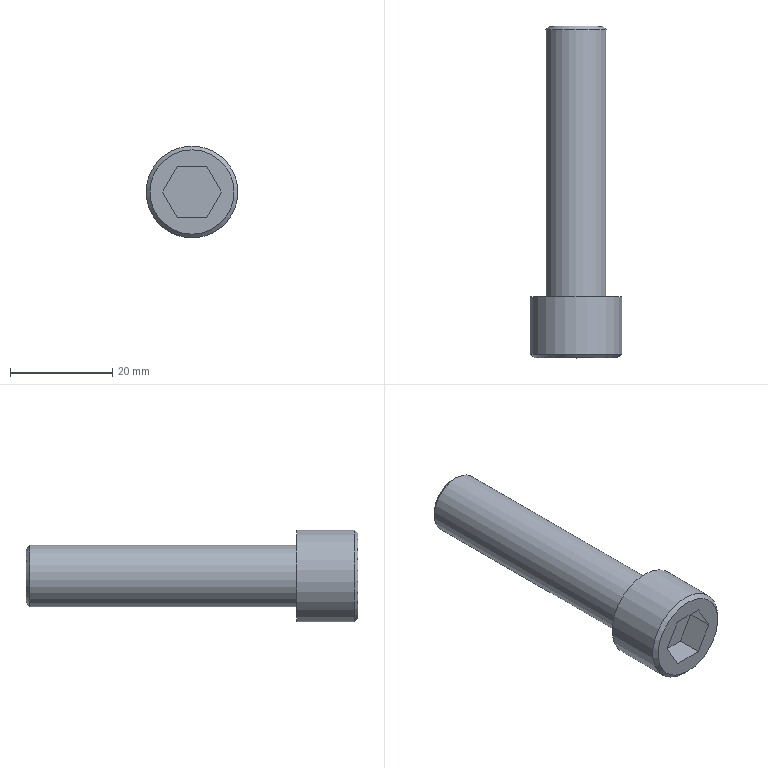Part | STEP file | solid 167 | 1 solid | 14 faces | box 18 x 65 x 18 mm | volume 8589 mm3 | plane 10 | cone 2 | cylinder 2 | commonest cylinder face diameters 12 x1 18 x1